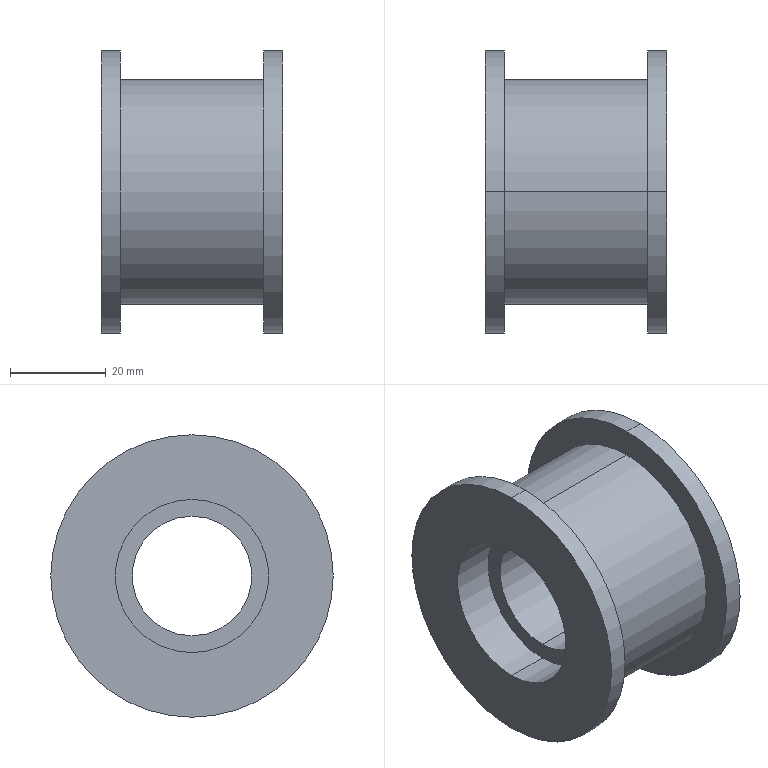Part | STEP file | PN_0041 (slide wheel) | 1 solid | 18 faces | box 38 x 59 x 59 mm | volume 49626 mm3 | cylinder 12 | plane 6 | commonest cylinder face diameters 32 x4 59 x4 25 x2 47 x2
STEP:
#1=CARTESIAN_POINT('',(0.,0.,0.));
#2=DIRECTION('',(0.,0.,1.));
#3=DIRECTION('',(1.,0.,0.));
#4=AXIS2_PLACEMENT_3D('',#1,#2,#3);
#5=CARTESIAN_POINT('',(9.,0.,16.));
#6=VERTEX_POINT('',#5);
#7=CARTESIAN_POINT('',(0.,0.,16.));
#8=VERTEX_POINT('',#7);
#9=CARTESIAN_POINT('',(9.,0.,16.));
#10=DIRECTION('',(-1.,0.,0.));
#11=VECTOR('',#10,1.);
#12=LINE('',#9,#11);
#13=CARTESIAN_POINT('',(9.,0.,0.));
#14=DIRECTION('',(-1.,0.,0.));
#15=DIRECTION('',(0.,0.,1.));
#16=AXIS2_PLACEMENT_3D('',#13,#14,#15);
#17=CYLINDRICAL_SURFACE('',#16,16.);
#18=CARTESIAN_POINT('',(6.283,0.));
#19=DIRECTION('',(0.,1.));
#20=VECTOR('',#19,1.);
#21=LINE('',#18,#20);
#22=(GEOMETRIC_REPRESENTATION_CONTEXT(2)PARAMETRIC_REPRESENTATION_CONTEXT()REPRESENTATION_CONTEXT('',''));
#23=DEFINITIONAL_REPRESENTATION('',(#21),#22);
#24=PCURVE('',#17,#23);
#25=CARTESIAN_POINT('',(9.,0.,0.));
#26=DIRECTION('',(-1.,0.,0.));
#27=DIRECTION('',(0.,0.,1.));
#28=AXIS2_PLACEMENT_3D('',#25,#26,#27);
#29=CYLINDRICAL_SURFACE('',#28,16.);
#30=CARTESIAN_POINT('',(0.,0.));
#31=DIRECTION('',(0.,1.));
#32=VECTOR('',#31,1.);
#33=LINE('',#30,#32);
#34=(GEOMETRIC_REPRESENTATION_CONTEXT(2)PARAMETRIC_REPRESENTATION_CONTEXT()REPRESENTATION_CONTEXT('',''));
#35=DEFINITIONAL_REPRESENTATION('',(#33),#34);
#36=PCURVE('',#29,#35);
#37=SURFACE_CURVE('',#12,(#24,#36),.PCURVE_S1.);
#38=EDGE_CURVE('',#6,#8,#37,.T.);
#39=ORIENTED_EDGE('',*,*,#38,.T.);
#40=CARTESIAN_POINT('',(0.,0.,-16.));
#41=VERTEX_POINT('',#40);
#42=CARTESIAN_POINT('',(0.,0.,0.));
#43=DIRECTION('',(-1.,0.,0.));
#44=DIRECTION('',(0.,0.,1.));
#45=AXIS2_PLACEMENT_3D('',#42,#43,#44);
#46=CIRCLE('',#45,16.);
#47=CARTESIAN_POINT('',(0.,9.));
#48=DIRECTION('',(1.,0.));
#49=VECTOR('',#48,1.);
#50=LINE('',#47,#49);
#51=(GEOMETRIC_REPRESENTATION_CONTEXT(2)PARAMETRIC_REPRESENTATION_CONTEXT()REPRESENTATION_CONTEXT('',''));
#52=DEFINITIONAL_REPRESENTATION('',(#50),#51);
#53=PCURVE('',#17,#52);
#54=CARTESIAN_POINT('',(0.,0.,0.));
#55=DIRECTION('',(1.,0.,0.));
#56=DIRECTION('',(0.,0.,-1.));
#57=AXIS2_PLACEMENT_3D('',#54,#55,#56);
#58=PLANE('',#57);
#59=CARTESIAN_POINT('',(-16.,0.));
#60=CARTESIAN_POINT('',(-16.,27.713));
#61=CARTESIAN_POINT('',(8.,13.856));
#62=CARTESIAN_POINT('',(32.,0.));
#63=CARTESIAN_POINT('',(8.,-13.856));
#64=CARTESIAN_POINT('',(-16.,-27.713));
#65=CARTESIAN_POINT('',(-16.,0.));
#66=(BOUNDED_CURVE()B_SPLINE_CURVE(2,(#59,#60,#61,#62,#63,#64,#65),.UNSPECIFIED.,.T.,.F.)B_SPLINE_CURVE_WITH_KNOTS((1,2,2,2,2,1),(-2.094,0.,2.094,4.189,6.283,8.378),.UNSPECIFIED.)CURVE()GEOMETRIC_REPRESENTATION_ITEM()RATIONAL_B_SPLINE_CURVE((1.,0.5,1.,0.5,1.,0.5,1.))REPRESENTATION_ITEM(''));
#67=(GEOMETRIC_REPRESENTATION_CONTEXT(2)PARAMETRIC_REPRESENTATION_CONTEXT()REPRESENTATION_CONTEXT('',''));
#68=DEFINITIONAL_REPRESENTATION('',(#66),#67);
#69=PCURVE('',#58,#68);
#70=SURFACE_CURVE('',#46,(#53,#69),.PCURVE_S1.);
#71=EDGE_CURVE('',#41,#8,#70,.T.);
#72=ORIENTED_EDGE('',*,*,#71,.F.);
#73=CARTESIAN_POINT('',(9.,0.,-16.));
#74=VERTEX_POINT('',#73);
#75=CARTESIAN_POINT('',(9.,0.,-16.));
#76=DIRECTION('',(-1.,0.,0.));
#77=VECTOR('',#76,1.);
#78=LINE('',#75,#77);
#79=CARTESIAN_POINT('',(3.142,0.));
#80=DIRECTION('',(0.,1.));
#81=VECTOR('',#80,1.);
#82=LINE('',#79,#81);
#83=(GEOMETRIC_REPRESENTATION_CONTEXT(2)PARAMETRIC_REPRESENTATION_CONTEXT()REPRESENTATION_CONTEXT('',''));
#84=DEFINITIONAL_REPRESENTATION('',(#82),#83);
#85=PCURVE('',#17,#84);
#86=CARTESIAN_POINT('',(3.142,0.));
#87=DIRECTION('',(0.,1.));
#88=VECTOR('',#87,1.);
#89=LINE('',#86,#88);
#90=(GEOMETRIC_REPRESENTATION_CONTEXT(2)PARAMETRIC_REPRESENTATION_CONTEXT()REPRESENTATION_CONTEXT('',''));
#91=DEFINITIONAL_REPRESENTATION('',(#89),#90);
#92=PCURVE('',#29,#91);
#93=SURFACE_CURVE('',#78,(#85,#92),.PCURVE_S1.);
#94=EDGE_CURVE('',#74,#41,#93,.T.);
#95=ORIENTED_EDGE('',*,*,#94,.F.);
#96=CARTESIAN_POINT('',(9.,0.,0.));
#97=DIRECTION('',(-1.,0.,0.));
#98=DIRECTION('',(0.,0.,1.));
#99=AXIS2_PLACEMENT_3D('',#96,#97,#98);
#100=CIRCLE('',#99,16.);
#101=CARTESIAN_POINT('',(0.,0.));
#102=DIRECTION('',(1.,0.));
#103=VECTOR('',#102,1.);
#104=LINE('',#101,#103);
#105=(GEOMETRIC_REPRESENTATION_CONTEXT(2)PARAMETRIC_REPRESENTATION_CONTEXT()REPRESENTATION_CONTEXT('',''));
#106=DEFINITIONAL_REPRESENTATION('',(#104),#105);
#107=PCURVE('',#17,#106);
#108=CARTESIAN_POINT('',(9.,0.,0.));
#109=DIRECTION('',(-1.,0.,0.));
#110=DIRECTION('',(0.,0.,1.));
#111=AXIS2_PLACEMENT_3D('',#108,#109,#110);
#112=PLANE('',#111);
#113=CARTESIAN_POINT('',(0.,0.));
#114=DIRECTION('',(1.,0.));
#115=AXIS2_PLACEMENT_2D('',#113,#114);
#116=CIRCLE('',#115,16.);
#117=(GEOMETRIC_REPRESENTATION_CONTEXT(2)PARAMETRIC_REPRESENTATION_CONTEXT()REPRESENTATION_CONTEXT('',''));
#118=DEFINITIONAL_REPRESENTATION('',(#116),#117);
#119=PCURVE('',#112,#118);
#120=SURFACE_CURVE('',#100,(#107,#119),.PCURVE_S1.);
#121=EDGE_CURVE('',#74,#6,#120,.T.);
#122=ORIENTED_EDGE('',*,*,#121,.T.);
#123=EDGE_LOOP('',(#39,#72,#95,#122));
#124=FACE_BOUND('',#123,.F.);
#125=ADVANCED_FACE('',(#124),#17,.F.);
#126=CARTESIAN_POINT('',(29.,0.,-16.));
#127=VERTEX_POINT('',#126);
#128=CARTESIAN_POINT('',(38.,0.,-16.));
#129=VERTEX_POINT('',#128);
#130=CARTESIAN_POINT('',(29.,0.,-16.));
#131=DIRECTION('',(1.,0.,0.));
#132=VECTOR('',#131,1.);
#133=LINE('',#130,#132);
#134=CARTESIAN_POINT('',(29.,0.,0.));
#135=DIRECTION('',(1.,0.,0.));
#136=DIRECTION('',(0.,0.,-1.));
#137=AXIS2_PLACEMENT_3D('',#134,#135,#136);
#138=CYLINDRICAL_SURFACE('',#137,16.);
#139=CARTESIAN_POINT('',(6.283,0.));
#140=DIRECTION('',(0.,1.));
#141=VECTOR('',#140,1.);
#142=LINE('',#139,#141);
#143=(GEOMETRIC_REPRESENTATION_CONTEXT(2)PARAMETRIC_REPRESENTATION_CONTEXT()REPRESENTATION_CONTEXT('',''));
#144=DEFINITIONAL_REPRESENTATION('',(#142),#143);
#145=PCURVE('',#138,#144);
#146=CARTESIAN_POINT('',(29.,0.,0.));
#147=DIRECTION('',(1.,0.,0.));
#148=DIRECTION('',(0.,0.,-1.));
#149=AXIS2_PLACEMENT_3D('',#146,#147,#148);
#150=CYLINDRICAL_SURFACE('',#149,16.);
#151=CARTESIAN_POINT('',(0.,0.));
#152=DIRECTION('',(0.,1.));
#153=VECTOR('',#152,1.);
#154=LINE('',#151,#153);
#155=(GEOMETRIC_REPRESENTATION_CONTEXT(2)PARAMETRIC_REPRESENTATION_CONTEXT()REPRESENTATION_CONTEXT('',''));
#156=DEFINITIONAL_REPRESENTATION('',(#154),#155);
#157=PCURVE('',#150,#156);
#158=SURFACE_CURVE('',#133,(#145,#157),.PCURVE_S1.);
#159=EDGE_CURVE('',#127,#129,#158,.T.);
#160=ORIENTED_EDGE('',*,*,#159,.T.);
#161=CARTESIAN_POINT('',(38.,0.,16.));
#162=VERTEX_POINT('',#161);
#163=CARTESIAN_POINT('',(38.,0.,0.));
#164=DIRECTION('',(1.,0.,0.));
#165=DIRECTION('',(0.,0.,-1.));
#166=AXIS2_PLACEMENT_3D('',#163,#164,#165);
#167=CIRCLE('',#166,16.);
#168=CARTESIAN_POINT('',(0.,9.));
#169=DIRECTION('',(1.,0.));
#170=VECTOR('',#169,1.);
#171=LINE('',#168,#170);
#172=(GEOMETRIC_REPRESENTATION_CONTEXT(2)PARAMETRIC_REPRESENTATION_CONTEXT()REPRESENTATION_CONTEXT('',''));
#173=DEFINITIONAL_REPRESENTATION('',(#171),#172);
#174=PCURVE('',#138,#173);
#175=CARTESIAN_POINT('',(38.,29.5,0.));
#176=DIRECTION('',(-1.,0.,0.));
#177=DIRECTION('',(0.,0.,1.));
#178=AXIS2_PLACEMENT_3D('',#175,#176,#177);
#179=PLANE('',#178);
#180=CARTESIAN_POINT('',(-16.,-29.5));
#181=CARTESIAN_POINT('',(-16.,-1.787));
#182=CARTESIAN_POINT('',(8.,-15.644));
#183=CARTESIAN_POINT('',(32.,-29.5));
#184=CARTESIAN_POINT('',(8.,-43.356));
#185=CARTESIAN_POINT('',(-16.,-57.213));
#186=CARTESIAN_POINT('',(-16.,-29.5));
#187=(BOUNDED_CURVE()B_SPLINE_CURVE(2,(#180,#181,#182,#183,#184,#185,#186),.UNSPECIFIED.,.T.,.F.)B_SPLINE_CURVE_WITH_KNOTS((1,2,2,2,2,1),(-2.094,0.,2.094,4.189,6.283,8.378),.UNSPECIFIED.)CURVE()GEOMETRIC_REPRESENTATION_ITEM()RATIONAL_B_SPLINE_CURVE((1.,0.5,1.,0.5,1.,0.5,1.))REPRESENTATION_ITEM(''));
#188=(GEOMETRIC_REPRESENTATION_CONTEXT(2)PARAMETRIC_REPRESENTATION_CONTEXT()REPRESENTATION_CONTEXT('',''));
#189=DEFINITIONAL_REPRESENTATION('',(#187),#188);
#190=PCURVE('',#179,#189);
#191=SURFACE_CURVE('',#167,(#174,#190),.PCURVE_S1.);
#192=EDGE_CURVE('',#162,#129,#191,.T.);
#193=ORIENTED_EDGE('',*,*,#192,.F.);
#194=CARTESIAN_POINT('',(29.,0.,16.));
#195=VERTEX_POINT('',#194);
#196=CARTESIAN_POINT('',(29.,0.,16.));
#197=DIRECTION('',(1.,0.,0.));
#198=VECTOR('',#197,1.);
#199=LINE('',#196,#198);
#200=CARTESIAN_POINT('',(3.142,0.));
#201=DIRECTION('',(0.,1.));
#202=VECTOR('',#201,1.);
#203=LINE('',#200,#202);
#204=(GEOMETRIC_REPRESENTATION_CONTEXT(2)PARAMETRIC_REPRESENTATION_CONTEXT()REPRESENTATION_CONTEXT('',''));
#205=DEFINITIONAL_REPRESENTATION('',(#203),#204);
#206=PCURVE('',#138,#205);
#207=CARTESIAN_POINT('',(3.142,0.));
#208=DIRECTION('',(0.,1.));
#209=VECTOR('',#208,1.);
#210=LINE('',#207,#209);
#211=(GEOMETRIC_REPRESENTATION_CONTEXT(2)PARAMETRIC_REPRESENTATION_CONTEXT()REPRESENTATION_CONTEXT('',''));
#212=DEFINITIONAL_REPRESENTATION('',(#210),#211);
#213=PCURVE('',#150,#212);
#214=SURFACE_CURVE('',#199,(#206,#213),.PCURVE_S1.);
#215=EDGE_CURVE('',#195,#162,#214,.T.);
#216=ORIENTED_EDGE('',*,*,#215,.F.);
#217=CARTESIAN_POINT('',(29.,0.,0.));
#218=DIRECTION('',(1.,0.,0.));
#219=DIRECTION('',(0.,0.,-1.));
#220=AXIS2_PLACEMENT_3D('',#217,#218,#219);
#221=CIRCLE('',#220,16.);
#222=CARTESIAN_POINT('',(0.,0.));
#223=DIRECTION('',(1.,0.));
#224=VECTOR('',#223,1.);
#225=LINE('',#222,#224);
#226=(GEOMETRIC_REPRESENTATION_CONTEXT(2)PARAMETRIC_REPRESENTATION_CONTEXT()REPRESENTATION_CONTEXT('',''));
#227=DEFINITIONAL_REPRESENTATION('',(#225),#226);
#228=PCURVE('',#138,#227);
#229=CARTESIAN_POINT('',(29.,0.,0.));
#230=DIRECTION('',(1.,0.,0.));
#231=DIRECTION('',(0.,0.,-1.));
#232=AXIS2_PLACEMENT_3D('',#229,#230,#231);
#233=PLANE('',#232);
#234=CARTESIAN_POINT('',(0.,0.));
#235=DIRECTION('',(1.,0.));
#236=AXIS2_PLACEMENT_2D('',#234,#235);
#237=CIRCLE('',#236,16.);
#238=(GEOMETRIC_REPRESENTATION_CONTEXT(2)PARAMETRIC_REPRESENTATION_CONTEXT()REPRESENTATION_CONTEXT('',''));
#239=DEFINITIONAL_REPRESENTATION('',(#237),#238);
#240=PCURVE('',#233,#239);
#241=SURFACE_CURVE('',#221,(#228,#240),.PCURVE_S1.);
#242=EDGE_CURVE('',#195,#127,#241,.T.);
#243=ORIENTED_EDGE('',*,*,#242,.T.);
#244=EDGE_LOOP('',(#160,#193,#216,#243));
#245=FACE_BOUND('',#244,.F.);
#246=ADVANCED_FACE('',(#245),#138,.F.);
#247=CARTESIAN_POINT('',(38.,0.,29.5));
#248=VERTEX_POINT('',#247);
#249=CARTESIAN_POINT('',(38.,0.,-29.5));
#250=VERTEX_POINT('',#249);
#251=CARTESIAN_POINT('',(38.,0.,0.));
#252=DIRECTION('',(-1.,0.,0.));
#253=DIRECTION('',(0.,0.,1.));
#254=AXIS2_PLACEMENT_3D('',#251,#252,#253);
#255=CIRCLE('',#254,29.5);
#256=CARTESIAN_POINT('',(0.,0.,0.));
#257=DIRECTION('',(-1.,0.,0.));
#258=DIRECTION('',(0.,0.,1.));
#259=AXIS2_PLACEMENT_3D('',#256,#257,#258);
#260=CYLINDRICAL_SURFACE('',#259,29.5);
#261=CARTESIAN_POINT('',(0.,-38.));
#262=DIRECTION('',(1.,0.));
#263=VECTOR('',#262,1.);
#264=LINE('',#261,#263);
#265=(GEOMETRIC_REPRESENTATION_CONTEXT(2)PARAMETRIC_REPRESENTATION_CONTEXT()REPRESENTATION_CONTEXT('',''));
#266=DEFINITIONAL_REPRESENTATION('',(#264),#265);
#267=PCURVE('',#260,#266);
#268=CARTESIAN_POINT('',(0.,-29.5));
#269=DIRECTION('',(1.,0.));
#270=AXIS2_PLACEMENT_2D('',#268,#269);
#271=CIRCLE('',#270,29.5);
#272=(GEOMETRIC_REPRESENTATION_CONTEXT(2)PARAMETRIC_REPRESENTATION_CONTEXT()REPRESENTATION_CONTEXT('',''));
#273=DEFINITIONAL_REPRESENTATION('',(#271),#272);
#274=PCURVE('',#179,#273);
#275=SURFACE_CURVE('',#255,(#267,#274),.PCURVE_S1.);
#276=EDGE_CURVE('',#248,#250,#275,.T.);
#277=ORIENTED_EDGE('',*,*,#276,.T.);
#278=CARTESIAN_POINT('',(34.,0.,-29.5));
#279=VERTEX_POINT('',#278);
#280=CARTESIAN_POINT('',(0.,0.,-29.5));
#281=DIRECTION('',(-1.,0.,0.));
#282=VECTOR('',#281,1.);
#283=LINE('',#280,#282);
#284=CARTESIAN_POINT('',(3.142,0.));
#285=DIRECTION('',(0.,1.));
#286=VECTOR('',#285,1.);
#287=LINE('',#284,#286);
#288=(GEOMETRIC_REPRESENTATION_CONTEXT(2)PARAMETRIC_REPRESENTATION_CONTEXT()REPRESENTATION_CONTEXT('',''));
#289=DEFINITIONAL_REPRESENTATION('',(#287),#288);
#290=PCURVE('',#260,#289);
#291=CARTESIAN_POINT('',(0.,0.,0.));
#292=DIRECTION('',(-1.,0.,0.));
#293=DIRECTION('',(0.,0.,1.));
#294=AXIS2_PLACEMENT_3D('',#291,#292,#293);
#295=CYLINDRICAL_SURFACE('',#294,29.5);
#296=CARTESIAN_POINT('',(3.142,0.));
#297=DIRECTION('',(0.,1.));
#298=VECTOR('',#297,1.);
#299=LINE('',#296,#298);
#300=(GEOMETRIC_REPRESENTATION_CONTEXT(2)PARAMETRIC_REPRESENTATION_CONTEXT()REPRESENTATION_CONTEXT('',''));
#301=DEFINITIONAL_REPRESENTATION('',(#299),#300);
#302=PCURVE('',#295,#301);
#303=SURFACE_CURVE('',#283,(#290,#302),.PCURVE_S1.);
#304=EDGE_CURVE('',#250,#279,#303,.T.);
#305=ORIENTED_EDGE('',*,*,#304,.T.);
#306=CARTESIAN_POINT('',(34.,0.,29.5));
#307=VERTEX_POINT('',#306);
#308=CARTESIAN_POINT('',(34.,0.,0.));
#309=DIRECTION('',(-1.,0.,0.));
#310=DIRECTION('',(0.,0.,1.));
#311=AXIS2_PLACEMENT_3D('',#308,#309,#310);
#312=CIRCLE('',#311,29.5);
#313=CARTESIAN_POINT('',(0.,-34.));
#314=DIRECTION('',(1.,0.));
#315=VECTOR('',#314,1.);
#316=LINE('',#313,#315);
#317=(GEOMETRIC_REPRESENTATION_CONTEXT(2)PARAMETRIC_REPRESENTATION_CONTEXT()REPRESENTATION_CONTEXT('',''));
#318=DEFINITIONAL_REPRESENTATION('',(#316),#317);
#319=PCURVE('',#260,#318);
#320=CARTESIAN_POINT('',(34.,23.5,0.));
#321=DIRECTION('',(1.,0.,0.));
#322=DIRECTION('',(0.,0.,-1.));
#323=AXIS2_PLACEMENT_3D('',#320,#321,#322);
#324=PLANE('',#323);
#325=CARTESIAN_POINT('',(-29.5,-23.5));
#326=CARTESIAN_POINT('',(-29.5,27.595));
#327=CARTESIAN_POINT('',(14.75,2.048));
#328=CARTESIAN_POINT('',(59.,-23.5));
#329=CARTESIAN_POINT('',(14.75,-49.048));
#330=CARTESIAN_POINT('',(-29.5,-74.595));
#331=CARTESIAN_POINT('',(-29.5,-23.5));
#332=(BOUNDED_CURVE()B_SPLINE_CURVE(2,(#325,#326,#327,#328,#329,#330,#331),.UNSPECIFIED.,.T.,.F.)B_SPLINE_CURVE_WITH_KNOTS((1,2,2,2,2,1),(-2.094,0.,2.094,4.189,6.283,8.378),.UNSPECIFIED.)CURVE()GEOMETRIC_REPRESENTATION_ITEM()RATIONAL_B_SPLINE_CURVE((1.,0.5,1.,0.5,1.,0.5,1.))REPRESENTATION_ITEM(''));
#333=(GEOMETRIC_REPRESENTATION_CONTEXT(2)PARAMETRIC_REPRESENTATION_CONTEXT()REPRESENTATION_CONTEXT('',''));
#334=DEFINITIONAL_REPRESENTATION('',(#332),#333);
#335=PCURVE('',#324,#334);
#336=SURFACE_CURVE('',#312,(#319,#335),.PCURVE_S1.);
#337=EDGE_CURVE('',#307,#279,#336,.T.);
#338=ORIENTED_EDGE('',*,*,#337,.F.);
#339=CARTESIAN_POINT('',(0.,0.,29.5));
#340=DIRECTION('',(-1.,0.,0.));
#341=VECTOR('',#340,1.);
#342=LINE('',#339,#341);
#343=CARTESIAN_POINT('',(0.,0.));
#344=DIRECTION('',(0.,1.));
#345=VECTOR('',#344,1.);
#346=LINE('',#343,#345);
#347=(GEOMETRIC_REPRESENTATION_CONTEXT(2)PARAMETRIC_REPRESENTATION_CONTEXT()REPRESENTATION_CONTEXT('',''));
#348=DEFINITIONAL_REPRESENTATION('',(#346),#347);
#349=PCURVE('',#260,#348);
#350=CARTESIAN_POINT('',(6.283,0.));
#351=DIRECTION('',(0.,1.));
#352=VECTOR('',#351,1.);
#353=LINE('',#350,#352);
#354=(GEOMETRIC_REPRESENTATION_CONTEXT(2)PARAMETRIC_REPRESENTATION_CONTEXT()REPRESENTATION_CONTEXT('',''));
#355=DEFINITIONAL_REPRESENTATION('',(#353),#354);
#356=PCURVE('',#295,#355);
#357=SURFACE_CURVE('',#342,(#349,#356),.PCURVE_S1.);
#358=EDGE_CURVE('',#248,#307,#357,.T.);
#359=ORIENTED_EDGE('',*,*,#358,.F.);
#360=EDGE_LOOP('',(#277,#305,#338,#359));
#361=FACE_BOUND('',#360,.T.);
#362=ADVANCED_FACE('',(#361),#260,.T.);
#363=CARTESIAN_POINT('',(34.,0.,23.5));
#364=VERTEX_POINT('',#363);
#365=CARTESIAN_POINT('',(34.,0.,-23.5));
#366=VERTEX_POINT('',#365);
#367=CARTESIAN_POINT('',(34.,0.,0.));
#368=DIRECTION('',(-1.,0.,0.));
#369=DIRECTION('',(0.,0.,1.));
#370=AXIS2_PLACEMENT_3D('',#367,#368,#369);
#371=CIRCLE('',#370,23.5);
#372=CARTESIAN_POINT('',(0.,0.,0.));
#373=DIRECTION('',(-1.,0.,0.));
#374=DIRECTION('',(0.,0.,1.));
#375=AXIS2_PLACEMENT_3D('',#372,#373,#374);
#376=CYLINDRICAL_SURFACE('',#375,23.5);
#377=CARTESIAN_POINT('',(0.,-34.));
#378=DIRECTION('',(1.,0.));
#379=VECTOR('',#378,1.);
#380=LINE('',#377,#379);
#381=(GEOMETRIC_REPRESENTATION_CONTEXT(2)PARAMETRIC_REPRESENTATION_CONTEXT()REPRESENTATION_CONTEXT('',''));
#382=DEFINITIONAL_REPRESENTATION('',(#380),#381);
#383=PCURVE('',#376,#382);
#384=CARTESIAN_POINT('',(-23.5,-23.5));
#385=CARTESIAN_POINT('',(-23.5,17.203));
#386=CARTESIAN_POINT('',(11.75,-3.148));
#387=CARTESIAN_POINT('',(47.,-23.5));
#388=CARTESIAN_POINT('',(11.75,-43.852));
#389=CARTESIAN_POINT('',(-23.5,-64.203));
#390=CARTESIAN_POINT('',(-23.5,-23.5));
#391=(BOUNDED_CURVE()B_SPLINE_CURVE(2,(#384,#385,#386,#387,#388,#389,#390),.UNSPECIFIED.,.T.,.F.)B_SPLINE_CURVE_WITH_KNOTS((1,2,2,2,2,1),(-2.094,0.,2.094,4.189,6.283,8.378),.UNSPECIFIED.)CURVE()GEOMETRIC_REPRESENTATION_ITEM()RATIONAL_B_SPLINE_CURVE((1.,0.5,1.,0.5,1.,0.5,1.))REPRESENTATION_ITEM(''));
#392=(GEOMETRIC_REPRESENTATION_CONTEXT(2)PARAMETRIC_REPRESENTATION_CONTEXT()REPRESENTATION_CONTEXT('',''));
#393=DEFINITIONAL_REPRESENTATION('',(#391),#392);
#394=PCURVE('',#324,#393);
#395=SURFACE_CURVE('',#371,(#383,#394),.PCURVE_S1.);
#396=EDGE_CURVE('',#364,#366,#395,.T.);
#397=ORIENTED_EDGE('',*,*,#396,.T.);
#398=CARTESIAN_POINT('',(4.,0.,-23.5));
#399=VERTEX_POINT('',#398);
#400=CARTESIAN_POINT('',(0.,0.,-23.5));
#401=DIRECTION('',(-1.,0.,0.));
#402=VECTOR('',#401,1.);
#403=LINE('',#400,#402);
#404=CARTESIAN_POINT('',(3.142,0.));
#405=DIRECTION('',(0.,1.));
#406=VECTOR('',#405,1.);
#407=LINE('',#404,#406);
#408=(GEOMETRIC_REPRESENTATION_CONTEXT(2)PARAMETRIC_REPRESENTATION_CONTEXT()REPRESENTATION_CONTEXT('',''));
#409=DEFINITIONAL_REPRESENTATION('',(#407),#408);
#410=PCURVE('',#376,#409);
#411=CARTESIAN_POINT('',(0.,0.,0.));
#412=DIRECTION('',(-1.,0.,0.));
#413=DIRECTION('',(0.,0.,1.));
#414=AXIS2_PLACEMENT_3D('',#411,#412,#413);
#415=CYLINDRICAL_SURFACE('',#414,23.5);
#416=CARTESIAN_POINT('',(3.142,0.));
#417=DIRECTION('',(0.,1.));
#418=VECTOR('',#417,1.);
#419=LINE('',#416,#418);
#420=(GEOMETRIC_REPRESENTATION_CONTEXT(2)PARAMETRIC_REPRESENTATION_CONTEXT()REPRESENTATION_CONTEXT('',''));
#421=DEFINITIONAL_REPRESENTATION('',(#419),#420);
#422=PCURVE('',#415,#421);
#423=SURFACE_CURVE('',#403,(#410,#422),.PCURVE_S1.);
#424=EDGE_CURVE('',#366,#399,#423,.T.);
#425=ORIENTED_EDGE('',*,*,#424,.T.);
#426=CARTESIAN_POINT('',(4.,0.,23.5));
#427=VERTEX_POINT('',#426);
#428=CARTESIAN_POINT('',(4.,0.,0.));
#429=DIRECTION('',(-1.,0.,0.));
#430=DIRECTION('',(0.,0.,1.));
#431=AXIS2_PLACEMENT_3D('',#428,#429,#430);
#432=CIRCLE('',#431,23.5);
#433=CARTESIAN_POINT('',(0.,-4.));
#434=DIRECTION('',(1.,0.));
#435=VECTOR('',#434,1.);
#436=LINE('',#433,#435);
#437=(GEOMETRIC_REPRESENTATION_CONTEXT(2)PARAMETRIC_REPRESENTATION_CONTEXT()REPRESENTATION_CONTEXT('',''));
#438=DEFINITIONAL_REPRESENTATION('',(#436),#437);
#439=PCURVE('',#376,#438);
#440=CARTESIAN_POINT('',(4.,29.5,0.));
#441=DIRECTION('',(-1.,0.,0.));
#442=DIRECTION('',(0.,0.,1.));
#443=AXIS2_PLACEMENT_3D('',#440,#441,#442);
#444=PLANE('',#443);
#445=CARTESIAN_POINT('',(0.,-29.5));
#446=DIRECTION('',(1.,0.));
#447=AXIS2_PLACEMENT_2D('',#445,#446);
#448=CIRCLE('',#447,23.5);
#449=(GEOMETRIC_REPRESENTATION_CONTEXT(2)PARAMETRIC_REPRESENTATION_CONTEXT()REPRESENTATION_CONTEXT('',''));
#450=DEFINITIONAL_REPRESENTATION('',(#448),#449);
#451=PCURVE('',#444,#450);
#452=SURFACE_CURVE('',#432,(#439,#451),.PCURVE_S1.);
#453=EDGE_CURVE('',#427,#399,#452,.T.);
#454=ORIENTED_EDGE('',*,*,#453,.F.);
#455=CARTESIAN_POINT('',(0.,0.,23.5));
#456=DIRECTION('',(-1.,0.,0.));
#457=VECTOR('',#456,1.);
#458=LINE('',#455,#457);
#459=CARTESIAN_POINT('',(0.,0.));
#460=DIRECTION('',(0.,1.));
#461=VECTOR('',#460,1.);
#462=LINE('',#459,#461);
#463=(GEOMETRIC_REPRESENTATION_CONTEXT(2)PARAMETRIC_REPRESENTATION_CONTEXT()REPRESENTATION_CONTEXT('',''));
#464=DEFINITIONAL_REPRESENTATION('',(#462),#463);
#465=PCURVE('',#376,#464);
#466=CARTESIAN_POINT('',(6.283,0.));
#467=DIRECTION('',(0.,1.));
#468=VECTOR('',#467,1.);
#469=LINE('',#466,#468);
#470=(GEOMETRIC_REPRESENTATION_CONTEXT(2)PARAMETRIC_REPRESENTATION_CONTEXT()REPRESENTATION_CONTEXT('',''));
#471=DEFINITIONAL_REPRESENTATION('',(#469),#470);
#472=PCURVE('',#415,#471);
#473=SURFACE_CURVE('',#458,(#465,#472),.PCURVE_S1.);
#474=EDGE_CURVE('',#364,#427,#473,.T.);
#475=ORIENTED_EDGE('',*,*,#474,.F.);
#476=EDGE_LOOP('',(#397,#425,#454,#475));
#477=FACE_BOUND('',#476,.T.);
#478=ADVANCED_FACE('',(#477),#376,.T.);
#479=CARTESIAN_POINT('',(4.,0.,29.5));
#480=VERTEX_POINT('',#479);
#481=CARTESIAN_POINT('',(4.,0.,-29.5));
#482=VERTEX_POINT('',#481);
#483=CARTESIAN_POINT('',(4.,0.,0.));
#484=DIRECTION('',(-1.,0.,0.));
#485=DIRECTION('',(0.,0.,1.));
#486=AXIS2_PLACEMENT_3D('',#483,#484,#485);
#487=CIRCLE('',#486,29.5);
#488=CARTESIAN_POINT('',(0.,0.,0.));
#489=DIRECTION('',(-1.,0.,0.));
#490=DIRECTION('',(0.,0.,1.));
#491=AXIS2_PLACEMENT_3D('',#488,#489,#490);
#492=CYLINDRICAL_SURFACE('',#491,29.5);
#493=CARTESIAN_POINT('',(0.,-4.));
#494=DIRECTION('',(1.,0.));
#495=VECTOR('',#494,1.);
#496=LINE('',#493,#495);
#497=(GEOMETRIC_REPRESENTATION_CONTEXT(2)PARAMETRIC_REPRESENTATION_CONTEXT()REPRESENTATION_CONTEXT('',''));
#498=DEFINITIONAL_REPRESENTATION('',(#496),#497);
#499=PCURVE('',#492,#498);
#500=CARTESIAN_POINT('',(0.,-29.5));
#501=DIRECTION('',(1.,0.));
#502=AXIS2_PLACEMENT_2D('',#500,#501);
#503=CIRCLE('',#502,29.5);
#504=(GEOMETRIC_REPRESENTATION_CONTEXT(2)PARAMETRIC_REPRESENTATION_CONTEXT()REPRESENTATION_CONTEXT('',''));
#505=DEFINITIONAL_REPRESENTATION('',(#503),#504);
#506=PCURVE('',#444,#505);
#507=SURFACE_CURVE('',#487,(#499,#506),.PCURVE_S1.);
#508=EDGE_CURVE('',#480,#482,#507,.T.);
#509=ORIENTED_EDGE('',*,*,#508,.T.);
#510=CARTESIAN_POINT('',(0.,0.,-29.5));
#511=VERTEX_POINT('',#510);
#512=CARTESIAN_POINT('',(0.,0.,-29.5));
#513=DIRECTION('',(-1.,0.,0.));
#514=VECTOR('',#513,1.);
#515=LINE('',#512,#514);
#516=CARTESIAN_POINT('',(3.142,0.));
#517=DIRECTION('',(0.,1.));
#518=VECTOR('',#517,1.);
#519=LINE('',#516,#518);
#520=(GEOMETRIC_REPRESENTATION_CONTEXT(2)PARAMETRIC_REPRESENTATION_CONTEXT()REPRESENTATION_CONTEXT('',''));
#521=DEFINITIONAL_REPRESENTATION('',(#519),#520);
#522=PCURVE('',#492,#521);
#523=CARTESIAN_POINT('',(0.,0.,0.));
#524=DIRECTION('',(-1.,0.,0.));
#525=DIRECTION('',(0.,0.,1.));
#526=AXIS2_PLACEMENT_3D('',#523,#524,#525);
#527=CYLINDRICAL_SURFACE('',#526,29.5);
#528=CARTESIAN_POINT('',(3.142,0.));
#529=DIRECTION('',(0.,1.));
#530=VECTOR('',#529,1.);
#531=LINE('',#528,#530);
#532=(GEOMETRIC_REPRESENTATION_CONTEXT(2)PARAMETRIC_REPRESENTATION_CONTEXT()REPRESENTATION_CONTEXT('',''));
#533=DEFINITIONAL_REPRESENTATION('',(#531),#532);
#534=PCURVE('',#527,#533);
#535=SURFACE_CURVE('',#515,(#522,#534),.PCURVE_S1.);
#536=EDGE_CURVE('',#482,#511,#535,.T.);
#537=ORIENTED_EDGE('',*,*,#536,.T.);
#538=CARTESIAN_POINT('',(0.,0.,29.5));
#539=VERTEX_POINT('',#538);
#540=CARTESIAN_POINT('',(0.,0.,0.));
#541=DIRECTION('',(-1.,0.,0.));
#542=DIRECTION('',(0.,0.,1.));
#543=AXIS2_PLACEMENT_3D('',#540,#541,#542);
#544=CIRCLE('',#543,29.5);
#545=CARTESIAN_POINT('',(0.,0.));
#546=DIRECTION('',(1.,0.));
#547=VECTOR('',#546,1.);
#548=LINE('',#545,#547);
#549=(GEOMETRIC_REPRESENTATION_CONTEXT(2)PARAMETRIC_REPRESENTATION_CONTEXT()REPRESENTATION_CONTEXT('',''));
#550=DEFINITIONAL_REPRESENTATION('',(#548),#549);
#551=PCURVE('',#492,#550);
#552=CARTESIAN_POINT('',(-29.5,0.));
#553=CARTESIAN_POINT('',(-29.5,51.095));
#554=CARTESIAN_POINT('',(14.75,25.548));
#555=CARTESIAN_POINT('',(59.,0.));
#556=CARTESIAN_POINT('',(14.75,-25.548));
#557=CARTESIAN_POINT('',(-29.5,-51.095));
#558=CARTESIAN_POINT('',(-29.5,0.));
#559=(BOUNDED_CURVE()B_SPLINE_CURVE(2,(#552,#553,#554,#555,#556,#557,#558),.UNSPECIFIED.,.T.,.F.)B_SPLINE_CURVE_WITH_KNOTS((1,2,2,2,2,1),(-2.094,0.,2.094,4.189,6.283,8.378),.UNSPECIFIED.)CURVE()GEOMETRIC_REPRESENTATION_ITEM()RATIONAL_B_SPLINE_CURVE((1.,0.5,1.,0.5,1.,0.5,1.))REPRESENTATION_ITEM(''));
#560=(GEOMETRIC_REPRESENTATION_CONTEXT(2)PARAMETRIC_REPRESENTATION_CONTEXT()REPRESENTATION_CONTEXT('',''));
#561=DEFINITIONAL_REPRESENTATION('',(#559),#560);
#562=PCURVE('',#58,#561);
#563=SURFACE_CURVE('',#544,(#551,#562),.PCURVE_S1.);
#564=EDGE_CURVE('',#539,#511,#563,.T.);
#565=ORIENTED_EDGE('',*,*,#564,.F.);
#566=CARTESIAN_POINT('',(0.,0.,29.5));
#567=DIRECTION('',(-1.,0.,0.));
#568=VECTOR('',#567,1.);
#569=LINE('',#566,#568);
#570=CARTESIAN_POINT('',(0.,0.));
#571=DIRECTION('',(0.,1.));
#572=VECTOR('',#571,1.);
#573=LINE('',#570,#572);
#574=(GEOMETRIC_REPRESENTATION_CONTEXT(2)PARAMETRIC_REPRESENTATION_CONTEXT()REPRESENTATION_CONTEXT('',''));
#575=DEFINITIONAL_REPRESENTATION('',(#573),#574);
#576=PCURVE('',#492,#575);
#577=CARTESIAN_POINT('',(6.283,0.));
#578=DIRECTION('',(0.,1.));
#579=VECTOR('',#578,1.);
#580=LINE('',#577,#579);
#581=(GEOMETRIC_REPRESENTATION_CONTEXT(2)PARAMETRIC_REPRESENTATION_CONTEXT()REPRESENTATION_CONTEXT('',''));
#582=DEFINITIONAL_REPRESENTATION('',(#580),#581);
#583=PCURVE('',#527,#582);
#584=SURFACE_CURVE('',#569,(#576,#583),.PCURVE_S1.);
#585=EDGE_CURVE('',#480,#539,#584,.T.);
#586=ORIENTED_EDGE('',*,*,#585,.F.);
#587=EDGE_LOOP('',(#509,#537,#565,#586));
#588=FACE_BOUND('',#587,.T.);
#589=ADVANCED_FACE('',(#588),#492,.T.);
#590=CARTESIAN_POINT('',(9.,0.,-12.5));
#591=VERTEX_POINT('',#590);
#592=CARTESIAN_POINT('',(29.,0.,-12.5));
#593=VERTEX_POINT('',#592);
#594=CARTESIAN_POINT('',(0.,0.,-12.5));
#595=DIRECTION('',(1.,0.,0.));
#596=VECTOR('',#595,1.);
#597=LINE('',#594,#596);
#598=CARTESIAN_POINT('',(0.,0.,0.));
#599=DIRECTION('',(1.,0.,0.));
#600=DIRECTION('',(0.,0.,-1.));
#601=AXIS2_PLACEMENT_3D('',#598,#599,#600);
#602=CYLINDRICAL_SURFACE('',#601,12.5);
#603=CARTESIAN_POINT('',(6.283,0.));
#604=DIRECTION('',(0.,1.));
#605=VECTOR('',#604,1.);
#606=LINE('',#603,#605);
#607=(GEOMETRIC_REPRESENTATION_CONTEXT(2)PARAMETRIC_REPRESENTATION_CONTEXT()REPRESENTATION_CONTEXT('',''));
#608=DEFINITIONAL_REPRESENTATION('',(#606),#607);
#609=PCURVE('',#602,#608);
#610=CARTESIAN_POINT('',(0.,0.,0.));
#611=DIRECTION('',(1.,0.,0.));
#612=DIRECTION('',(0.,0.,-1.));
#613=AXIS2_PLACEMENT_3D('',#610,#611,#612);
#614=CYLINDRICAL_SURFACE('',#613,12.5);
#615=CARTESIAN_POINT('',(0.,0.));
#616=DIRECTION('',(0.,1.));
#617=VECTOR('',#616,1.);
#618=LINE('',#615,#617);
#619=(GEOMETRIC_REPRESENTATION_CONTEXT(2)PARAMETRIC_REPRESENTATION_CONTEXT()REPRESENTATION_CONTEXT('',''));
#620=DEFINITIONAL_REPRESENTATION('',(#618),#619);
#621=PCURVE('',#614,#620);
#622=SURFACE_CURVE('',#597,(#609,#621),.PCURVE_S1.);
#623=EDGE_CURVE('',#591,#593,#622,.T.);
#624=ORIENTED_EDGE('',*,*,#623,.T.);
#625=CARTESIAN_POINT('',(29.,0.,12.5));
#626=VERTEX_POINT('',#625);
#627=CARTESIAN_POINT('',(29.,0.,0.));
#628=DIRECTION('',(-1.,0.,0.));
#629=DIRECTION('',(0.,0.,-1.));
#630=AXIS2_PLACEMENT_3D('',#627,#628,#629);
#631=CIRCLE('',#630,12.5);
#632=CARTESIAN_POINT('',(6.283,29.));
#633=DIRECTION('',(-1.,0.));
#634=VECTOR('',#633,1.);
#635=LINE('',#632,#634);
#636=(GEOMETRIC_REPRESENTATION_CONTEXT(2)PARAMETRIC_REPRESENTATION_CONTEXT()REPRESENTATION_CONTEXT('',''));
#637=DEFINITIONAL_REPRESENTATION('',(#635),#636);
#638=PCURVE('',#602,#637);
#639=CARTESIAN_POINT('',(12.5,0.));
#640=CARTESIAN_POINT('',(12.5,-21.651));
#641=CARTESIAN_POINT('',(-6.25,-10.825));
#642=CARTESIAN_POINT('',(-25.,0.));
#643=CARTESIAN_POINT('',(-6.25,10.825));
#644=CARTESIAN_POINT('',(12.5,21.651));
#645=CARTESIAN_POINT('',(12.5,0.));
#646=(BOUNDED_CURVE()B_SPLINE_CURVE(2,(#639,#640,#641,#642,#643,#644,#645),.UNSPECIFIED.,.T.,.F.)B_SPLINE_CURVE_WITH_KNOTS((1,2,2,2,2,1),(-2.094,0.,2.094,4.189,6.283,8.378),.UNSPECIFIED.)CURVE()GEOMETRIC_REPRESENTATION_ITEM()RATIONAL_B_SPLINE_CURVE((1.,0.5,1.,0.5,1.,0.5,1.))REPRESENTATION_ITEM(''));
#647=(GEOMETRIC_REPRESENTATION_CONTEXT(2)PARAMETRIC_REPRESENTATION_CONTEXT()REPRESENTATION_CONTEXT('',''));
#648=DEFINITIONAL_REPRESENTATION('',(#646),#647);
#649=PCURVE('',#233,#648);
#650=SURFACE_CURVE('',#631,(#638,#649),.PCURVE_S1.);
#651=EDGE_CURVE('',#593,#626,#650,.T.);
#652=ORIENTED_EDGE('',*,*,#651,.T.);
#653=CARTESIAN_POINT('',(9.,0.,12.5));
#654=VERTEX_POINT('',#653);
#655=CARTESIAN_POINT('',(0.,0.,12.5));
#656=DIRECTION('',(1.,0.,0.));
#657=VECTOR('',#656,1.);
#658=LINE('',#655,#657);
#659=CARTESIAN_POINT('',(3.142,0.));
#660=DIRECTION('',(0.,1.));
#661=VECTOR('',#660,1.);
#662=LINE('',#659,#661);
#663=(GEOMETRIC_REPRESENTATION_CONTEXT(2)PARAMETRIC_REPRESENTATION_CONTEXT()REPRESENTATION_CONTEXT('',''));
#664=DEFINITIONAL_REPRESENTATION('',(#662),#663);
#665=PCURVE('',#602,#664);
#666=CARTESIAN_POINT('',(3.142,0.));
#667=DIRECTION('',(0.,1.));
#668=VECTOR('',#667,1.);
#669=LINE('',#666,#668);
#670=(GEOMETRIC_REPRESENTATION_CONTEXT(2)PARAMETRIC_REPRESENTATION_CONTEXT()REPRESENTATION_CONTEXT('',''));
#671=DEFINITIONAL_REPRESENTATION('',(#669),#670);
#672=PCURVE('',#614,#671);
#673=SURFACE_CURVE('',#658,(#665,#672),.PCURVE_S1.);
#674=EDGE_CURVE('',#654,#626,#673,.T.);
#675=ORIENTED_EDGE('',*,*,#674,.F.);
#676=CARTESIAN_POINT('',(9.,0.,0.));
#677=DIRECTION('',(1.,0.,0.));
#678=DIRECTION('',(0.,0.,1.));
#679=AXIS2_PLACEMENT_3D('',#676,#677,#678);
#680=CIRCLE('',#679,12.5);
#681=CARTESIAN_POINT('',(3.142,9.));
#682=DIRECTION('',(1.,0.));
#683=VECTOR('',#682,1.);
#684=LINE('',#681,#683);
#685=(GEOMETRIC_REPRESENTATION_CONTEXT(2)PARAMETRIC_REPRESENTATION_CONTEXT()REPRESENTATION_CONTEXT('',''));
#686=DEFINITIONAL_REPRESENTATION('',(#684),#685);
#687=PCURVE('',#602,#686);
#688=CARTESIAN_POINT('',(12.5,0.));
#689=CARTESIAN_POINT('',(12.5,-21.651));
#690=CARTESIAN_POINT('',(-6.25,-10.825));
#691=CARTESIAN_POINT('',(-25.,0.));
#692=CARTESIAN_POINT('',(-6.25,10.825));
#693=CARTESIAN_POINT('',(12.5,21.651));
#694=CARTESIAN_POINT('',(12.5,0.));
#695=(BOUNDED_CURVE()B_SPLINE_CURVE(2,(#688,#689,#690,#691,#692,#693,#694),.UNSPECIFIED.,.T.,.F.)B_SPLINE_CURVE_WITH_KNOTS((1,2,2,2,2,1),(-2.094,0.,2.094,4.189,6.283,8.378),.UNSPECIFIED.)CURVE()GEOMETRIC_REPRESENTATION_ITEM()RATIONAL_B_SPLINE_CURVE((1.,0.5,1.,0.5,1.,0.5,1.))REPRESENTATION_ITEM(''));
#696=(GEOMETRIC_REPRESENTATION_CONTEXT(2)PARAMETRIC_REPRESENTATION_CONTEXT()REPRESENTATION_CONTEXT('',''));
#697=DEFINITIONAL_REPRESENTATION('',(#695),#696);
#698=PCURVE('',#112,#697);
#699=SURFACE_CURVE('',#680,(#687,#698),.PCURVE_S1.);
#700=EDGE_CURVE('',#654,#591,#699,.T.);
#701=ORIENTED_EDGE('',*,*,#700,.T.);
#702=EDGE_LOOP('',(#624,#652,#675,#701));
#703=FACE_BOUND('',#702,.F.);
#704=ADVANCED_FACE('',(#703),#602,.F.);
#705=CARTESIAN_POINT('',(29.,0.,0.));
#706=DIRECTION('',(-1.,0.,0.));
#707=DIRECTION('',(0.,0.,-1.));
#708=AXIS2_PLACEMENT_3D('',#705,#706,#707);
#709=CIRCLE('',#708,12.5);
#710=CARTESIAN_POINT('',(6.283,29.));
#711=DIRECTION('',(-1.,0.));
#712=VECTOR('',#711,1.);
#713=LINE('',#710,#712);
#714=(GEOMETRIC_REPRESENTATION_CONTEXT(2)PARAMETRIC_REPRESENTATION_CONTEXT()REPRESENTATION_CONTEXT('',''));
#715=DEFINITIONAL_REPRESENTATION('',(#713),#714);
#716=PCURVE('',#614,#715);
#717=CARTESIAN_POINT('',(12.5,0.));
#718=CARTESIAN_POINT('',(12.5,-21.651));
#719=CARTESIAN_POINT('',(-6.25,-10.825));
#720=CARTESIAN_POINT('',(-25.,0.));
#721=CARTESIAN_POINT('',(-6.25,10.825));
#722=CARTESIAN_POINT('',(12.5,21.651));
#723=CARTESIAN_POINT('',(12.5,0.));
#724=(BOUNDED_CURVE()B_SPLINE_CURVE(2,(#717,#718,#719,#720,#721,#722,#723),.UNSPECIFIED.,.T.,.F.)B_SPLINE_CURVE_WITH_KNOTS((1,2,2,2,2,1),(-2.094,0.,2.094,4.189,6.283,8.378),.UNSPECIFIED.)CURVE()GEOMETRIC_REPRESENTATION_ITEM()RATIONAL_B_SPLINE_CURVE((1.,0.5,1.,0.5,1.,0.5,1.))REPRESENTATION_ITEM(''));
#725=(GEOMETRIC_REPRESENTATION_CONTEXT(2)PARAMETRIC_REPRESENTATION_CONTEXT()REPRESENTATION_CONTEXT('',''));
#726=DEFINITIONAL_REPRESENTATION('',(#724),#725);
#727=PCURVE('',#233,#726);
#728=SURFACE_CURVE('',#709,(#716,#727),.PCURVE_S1.);
#729=EDGE_CURVE('',#626,#593,#728,.T.);
#730=ORIENTED_EDGE('',*,*,#729,.T.);
#731=ORIENTED_EDGE('',*,*,#623,.F.);
#732=CARTESIAN_POINT('',(9.,0.,0.));
#733=DIRECTION('',(1.,0.,0.));
#734=DIRECTION('',(0.,0.,1.));
#735=AXIS2_PLACEMENT_3D('',#732,#733,#734);
#736=CIRCLE('',#735,12.5);
#737=CARTESIAN_POINT('',(-3.142,9.));
#738=DIRECTION('',(1.,0.));
#739=VECTOR('',#738,1.);
#740=LINE('',#737,#739);
#741=(GEOMETRIC_REPRESENTATION_CONTEXT(2)PARAMETRIC_REPRESENTATION_CONTEXT()REPRESENTATION_CONTEXT('',''));
#742=DEFINITIONAL_REPRESENTATION('',(#740),#741);
#743=PCURVE('',#614,#742);
#744=CARTESIAN_POINT('',(12.5,0.));
#745=CARTESIAN_POINT('',(12.5,-21.651));
#746=CARTESIAN_POINT('',(-6.25,-10.825));
#747=CARTESIAN_POINT('',(-25.,0.));
#748=CARTESIAN_POINT('',(-6.25,10.825));
#749=CARTESIAN_POINT('',(12.5,21.651));
#750=CARTESIAN_POINT('',(12.5,0.));
#751=(BOUNDED_CURVE()B_SPLINE_CURVE(2,(#744,#745,#746,#747,#748,#749,#750),.UNSPECIFIED.,.T.,.F.)B_SPLINE_CURVE_WITH_KNOTS((1,2,2,2,2,1),(-2.094,0.,2.094,4.189,6.283,8.378),.UNSPECIFIED.)CURVE()GEOMETRIC_REPRESENTATION_ITEM()RATIONAL_B_SPLINE_CURVE((1.,0.5,1.,0.5,1.,0.5,1.))REPRESENTATION_ITEM(''));
#752=(GEOMETRIC_REPRESENTATION_CONTEXT(2)PARAMETRIC_REPRESENTATION_CONTEXT()REPRESENTATION_CONTEXT('',''));
#753=DEFINITIONAL_REPRESENTATION('',(#751),#752);
#754=PCURVE('',#112,#753);
#755=SURFACE_CURVE('',#736,(#743,#754),.PCURVE_S1.);
#756=EDGE_CURVE('',#591,#654,#755,.T.);
#757=ORIENTED_EDGE('',*,*,#756,.T.);
#758=ORIENTED_EDGE('',*,*,#674,.T.);
#759=EDGE_LOOP('',(#730,#731,#757,#758));
#760=FACE_BOUND('',#759,.F.);
#761=ADVANCED_FACE('',(#760),#614,.F.);
#762=CARTESIAN_POINT('',(0.,0.,0.));
#763=DIRECTION('',(-1.,0.,0.));
#764=DIRECTION('',(0.,0.,1.));
#765=AXIS2_PLACEMENT_3D('',#762,#763,#764);
#766=CIRCLE('',#765,16.);
#767=CARTESIAN_POINT('',(-16.,0.));
#768=CARTESIAN_POINT('',(-16.,27.713));
#769=CARTESIAN_POINT('',(8.,13.856));
#770=CARTESIAN_POINT('',(32.,0.));
#771=CARTESIAN_POINT('',(8.,-13.856));
#772=CARTESIAN_POINT('',(-16.,-27.713));
#773=CARTESIAN_POINT('',(-16.,0.));
#774=(BOUNDED_CURVE()B_SPLINE_CURVE(2,(#767,#768,#769,#770,#771,#772,#773),.UNSPECIFIED.,.T.,.F.)B_SPLINE_CURVE_WITH_KNOTS((1,2,2,2,2,1),(-2.094,0.,2.094,4.189,6.283,8.378),.UNSPECIFIED.)CURVE()GEOMETRIC_REPRESENTATION_ITEM()RATIONAL_B_SPLINE_CURVE((1.,0.5,1.,0.5,1.,0.5,1.))REPRESENTATION_ITEM(''));
#775=(GEOMETRIC_REPRESENTATION_CONTEXT(2)PARAMETRIC_REPRESENTATION_CONTEXT()REPRESENTATION_CONTEXT('',''));
#776=DEFINITIONAL_REPRESENTATION('',(#774),#775);
#777=PCURVE('',#58,#776);
#778=CARTESIAN_POINT('',(0.,9.));
#779=DIRECTION('',(1.,0.));
#780=VECTOR('',#779,1.);
#781=LINE('',#778,#780);
#782=(GEOMETRIC_REPRESENTATION_CONTEXT(2)PARAMETRIC_REPRESENTATION_CONTEXT()REPRESENTATION_CONTEXT('',''));
#783=DEFINITIONAL_REPRESENTATION('',(#781),#782);
#784=PCURVE('',#29,#783);
#785=SURFACE_CURVE('',#766,(#777,#784),.PCURVE_S1.);
#786=EDGE_CURVE('',#8,#41,#785,.T.);
#787=ORIENTED_EDGE('',*,*,#786,.F.);
#788=ORIENTED_EDGE('',*,*,#71,.F.);
#789=EDGE_LOOP('',(#787,#788));
#790=FACE_BOUND('',#789,.T.);
#791=ORIENTED_EDGE('',*,*,#564,.T.);
#792=CARTESIAN_POINT('',(0.,0.,0.));
#793=DIRECTION('',(-1.,0.,0.));
#794=DIRECTION('',(0.,0.,1.));
#795=AXIS2_PLACEMENT_3D('',#792,#793,#794);
#796=CIRCLE('',#795,29.5);
#797=CARTESIAN_POINT('',(-29.5,0.));
#798=CARTESIAN_POINT('',(-29.5,51.095));
#799=CARTESIAN_POINT('',(14.75,25.548));
#800=CARTESIAN_POINT('',(59.,0.));
#801=CARTESIAN_POINT('',(14.75,-25.548));
#802=CARTESIAN_POINT('',(-29.5,-51.095));
#803=CARTESIAN_POINT('',(-29.5,0.));
#804=(BOUNDED_CURVE()B_SPLINE_CURVE(2,(#797,#798,#799,#800,#801,#802,#803),.UNSPECIFIED.,.T.,.F.)B_SPLINE_CURVE_WITH_KNOTS((1,2,2,2,2,1),(-2.094,0.,2.094,4.189,6.283,8.378),.UNSPECIFIED.)CURVE()GEOMETRIC_REPRESENTATION_ITEM()RATIONAL_B_SPLINE_CURVE((1.,0.5,1.,0.5,1.,0.5,1.))REPRESENTATION_ITEM(''));
#805=(GEOMETRIC_REPRESENTATION_CONTEXT(2)PARAMETRIC_REPRESENTATION_CONTEXT()REPRESENTATION_CONTEXT('',''));
#806=DEFINITIONAL_REPRESENTATION('',(#804),#805);
#807=PCURVE('',#58,#806);
#808=CARTESIAN_POINT('',(0.,0.));
#809=DIRECTION('',(1.,0.));
#810=VECTOR('',#809,1.);
#811=LINE('',#808,#810);
#812=(GEOMETRIC_REPRESENTATION_CONTEXT(2)PARAMETRIC_REPRESENTATION_CONTEXT()REPRESENTATION_CONTEXT('',''));
#813=DEFINITIONAL_REPRESENTATION('',(#811),#812);
#814=PCURVE('',#527,#813);
#815=SURFACE_CURVE('',#796,(#807,#814),.PCURVE_S1.);
#816=EDGE_CURVE('',#511,#539,#815,.T.);
#817=ORIENTED_EDGE('',*,*,#816,.T.);
#818=EDGE_LOOP('',(#791,#817));
#819=FACE_BOUND('',#818,.T.);
#820=ADVANCED_FACE('',(#790,#819),#58,.F.);
#821=ORIENTED_EDGE('',*,*,#536,.F.);
#822=CARTESIAN_POINT('',(4.,0.,0.));
#823=DIRECTION('',(-1.,0.,0.));
#824=DIRECTION('',(0.,0.,1.));
#825=AXIS2_PLACEMENT_3D('',#822,#823,#824);
#826=CIRCLE('',#825,29.5);
#827=CARTESIAN_POINT('',(0.,-4.));
#828=DIRECTION('',(1.,0.));
#829=VECTOR('',#828,1.);
#830=LINE('',#827,#829);
#831=(GEOMETRIC_REPRESENTATION_CONTEXT(2)PARAMETRIC_REPRESENTATION_CONTEXT()REPRESENTATION_CONTEXT('',''));
#832=DEFINITIONAL_REPRESENTATION('',(#830),#831);
#833=PCURVE('',#527,#832);
#834=CARTESIAN_POINT('',(0.,-29.5));
#835=DIRECTION('',(1.,0.));
#836=AXIS2_PLACEMENT_2D('',#834,#835);
#837=CIRCLE('',#836,29.5);
#838=(GEOMETRIC_REPRESENTATION_CONTEXT(2)PARAMETRIC_REPRESENTATION_CONTEXT()REPRESENTATION_CONTEXT('',''));
#839=DEFINITIONAL_REPRESENTATION('',(#837),#838);
#840=PCURVE('',#444,#839);
#841=SURFACE_CURVE('',#826,(#833,#840),.PCURVE_S1.);
#842=EDGE_CURVE('',#482,#480,#841,.T.);
#843=ORIENTED_EDGE('',*,*,#842,.T.);
#844=ORIENTED_EDGE('',*,*,#585,.T.);
#845=ORIENTED_EDGE('',*,*,#816,.F.);
#846=EDGE_LOOP('',(#821,#843,#844,#845));
#847=FACE_BOUND('',#846,.T.);
#848=ADVANCED_FACE('',(#847),#527,.T.);
#849=ORIENTED_EDGE('',*,*,#508,.F.);
#850=ORIENTED_EDGE('',*,*,#842,.F.);
#851=EDGE_LOOP('',(#849,#850));
#852=FACE_BOUND('',#851,.T.);
#853=ORIENTED_EDGE('',*,*,#453,.T.);
#854=CARTESIAN_POINT('',(4.,0.,0.));
#855=DIRECTION('',(-1.,0.,0.));
#856=DIRECTION('',(0.,0.,1.));
#857=AXIS2_PLACEMENT_3D('',#854,#855,#856);
#858=CIRCLE('',#857,23.5);
#859=CARTESIAN_POINT('',(0.,-29.5));
#860=DIRECTION('',(1.,0.));
#861=AXIS2_PLACEMENT_2D('',#859,#860);
#862=CIRCLE('',#861,23.5);
#863=(GEOMETRIC_REPRESENTATION_CONTEXT(2)PARAMETRIC_REPRESENTATION_CONTEXT()REPRESENTATION_CONTEXT('',''));
#864=DEFINITIONAL_REPRESENTATION('',(#862),#863);
#865=PCURVE('',#444,#864);
#866=CARTESIAN_POINT('',(0.,-4.));
#867=DIRECTION('',(1.,0.));
#868=VECTOR('',#867,1.);
#869=LINE('',#866,#868);
#870=(GEOMETRIC_REPRESENTATION_CONTEXT(2)PARAMETRIC_REPRESENTATION_CONTEXT()REPRESENTATION_CONTEXT('',''));
#871=DEFINITIONAL_REPRESENTATION('',(#869),#870);
#872=PCURVE('',#415,#871);
#873=SURFACE_CURVE('',#858,(#865,#872),.PCURVE_S1.);
#874=EDGE_CURVE('',#399,#427,#873,.T.);
#875=ORIENTED_EDGE('',*,*,#874,.T.);
#876=EDGE_LOOP('',(#853,#875));
#877=FACE_BOUND('',#876,.T.);
#878=ADVANCED_FACE('',(#852,#877),#444,.F.);
#879=ORIENTED_EDGE('',*,*,#424,.F.);
#880=CARTESIAN_POINT('',(34.,0.,0.));
#881=DIRECTION('',(-1.,0.,0.));
#882=DIRECTION('',(0.,0.,1.));
#883=AXIS2_PLACEMENT_3D('',#880,#881,#882);
#884=CIRCLE('',#883,23.5);
#885=CARTESIAN_POINT('',(0.,-34.));
#886=DIRECTION('',(1.,0.));
#887=VECTOR('',#886,1.);
#888=LINE('',#885,#887);
#889=(GEOMETRIC_REPRESENTATION_CONTEXT(2)PARAMETRIC_REPRESENTATION_CONTEXT()REPRESENTATION_CONTEXT('',''));
#890=DEFINITIONAL_REPRESENTATION('',(#888),#889);
#891=PCURVE('',#415,#890);
#892=CARTESIAN_POINT('',(-23.5,-23.5));
#893=CARTESIAN_POINT('',(-23.5,17.203));
#894=CARTESIAN_POINT('',(11.75,-3.148));
#895=CARTESIAN_POINT('',(47.,-23.5));
#896=CARTESIAN_POINT('',(11.75,-43.852));
#897=CARTESIAN_POINT('',(-23.5,-64.203));
#898=CARTESIAN_POINT('',(-23.5,-23.5));
#899=(BOUNDED_CURVE()B_SPLINE_CURVE(2,(#892,#893,#894,#895,#896,#897,#898),.UNSPECIFIED.,.T.,.F.)B_SPLINE_CURVE_WITH_KNOTS((1,2,2,2,2,1),(-2.094,0.,2.094,4.189,6.283,8.378),.UNSPECIFIED.)CURVE()GEOMETRIC_REPRESENTATION_ITEM()RATIONAL_B_SPLINE_CURVE((1.,0.5,1.,0.5,1.,0.5,1.))REPRESENTATION_ITEM(''));
#900=(GEOMETRIC_REPRESENTATION_CONTEXT(2)PARAMETRIC_REPRESENTATION_CONTEXT()REPRESENTATION_CONTEXT('',''));
#901=DEFINITIONAL_REPRESENTATION('',(#899),#900);
#902=PCURVE('',#324,#901);
#903=SURFACE_CURVE('',#884,(#891,#902),.PCURVE_S1.);
#904=EDGE_CURVE('',#366,#364,#903,.T.);
#905=ORIENTED_EDGE('',*,*,#904,.T.);
#906=ORIENTED_EDGE('',*,*,#474,.T.);
#907=ORIENTED_EDGE('',*,*,#874,.F.);
#908=EDGE_LOOP('',(#879,#905,#906,#907));
#909=FACE_BOUND('',#908,.T.);
#910=ADVANCED_FACE('',(#909),#415,.T.);
#911=ORIENTED_EDGE('',*,*,#396,.F.);
#912=ORIENTED_EDGE('',*,*,#904,.F.);
#913=EDGE_LOOP('',(#911,#912));
#914=FACE_BOUND('',#913,.T.);
#915=ORIENTED_EDGE('',*,*,#337,.T.);
#916=CARTESIAN_POINT('',(34.,0.,0.));
#917=DIRECTION('',(-1.,0.,0.));
#918=DIRECTION('',(0.,0.,1.));
#919=AXIS2_PLACEMENT_3D('',#916,#917,#918);
#920=CIRCLE('',#919,29.5);
#921=CARTESIAN_POINT('',(-29.5,-23.5));
#922=CARTESIAN_POINT('',(-29.5,27.595));
#923=CARTESIAN_POINT('',(14.75,2.048));
#924=CARTESIAN_POINT('',(59.,-23.5));
#925=CARTESIAN_POINT('',(14.75,-49.048));
#926=CARTESIAN_POINT('',(-29.5,-74.595));
#927=CARTESIAN_POINT('',(-29.5,-23.5));
#928=(BOUNDED_CURVE()B_SPLINE_CURVE(2,(#921,#922,#923,#924,#925,#926,#927),.UNSPECIFIED.,.T.,.F.)B_SPLINE_CURVE_WITH_KNOTS((1,2,2,2,2,1),(-2.094,0.,2.094,4.189,6.283,8.378),.UNSPECIFIED.)CURVE()GEOMETRIC_REPRESENTATION_ITEM()RATIONAL_B_SPLINE_CURVE((1.,0.5,1.,0.5,1.,0.5,1.))REPRESENTATION_ITEM(''));
#929=(GEOMETRIC_REPRESENTATION_CONTEXT(2)PARAMETRIC_REPRESENTATION_CONTEXT()REPRESENTATION_CONTEXT('',''));
#930=DEFINITIONAL_REPRESENTATION('',(#928),#929);
#931=PCURVE('',#324,#930);
#932=CARTESIAN_POINT('',(0.,-34.));
#933=DIRECTION('',(1.,0.));
#934=VECTOR('',#933,1.);
#935=LINE('',#932,#934);
#936=(GEOMETRIC_REPRESENTATION_CONTEXT(2)PARAMETRIC_REPRESENTATION_CONTEXT()REPRESENTATION_CONTEXT('',''));
#937=DEFINITIONAL_REPRESENTATION('',(#935),#936);
#938=PCURVE('',#295,#937);
#939=SURFACE_CURVE('',#920,(#931,#938),.PCURVE_S1.);
#940=EDGE_CURVE('',#279,#307,#939,.T.);
#941=ORIENTED_EDGE('',*,*,#940,.T.);
#942=EDGE_LOOP('',(#915,#941));
#943=FACE_BOUND('',#942,.T.);
#944=ADVANCED_FACE('',(#914,#943),#324,.F.);
#945=ORIENTED_EDGE('',*,*,#304,.F.);
#946=CARTESIAN_POINT('',(38.,0.,0.));
#947=DIRECTION('',(-1.,0.,0.));
#948=DIRECTION('',(0.,0.,1.));
#949=AXIS2_PLACEMENT_3D('',#946,#947,#948);
#950=CIRCLE('',#949,29.5);
#951=CARTESIAN_POINT('',(0.,-38.));
#952=DIRECTION('',(1.,0.));
#953=VECTOR('',#952,1.);
#954=LINE('',#951,#953);
#955=(GEOMETRIC_REPRESENTATION_CONTEXT(2)PARAMETRIC_REPRESENTATION_CONTEXT()REPRESENTATION_CONTEXT('',''));
#956=DEFINITIONAL_REPRESENTATION('',(#954),#955);
#957=PCURVE('',#295,#956);
#958=CARTESIAN_POINT('',(0.,-29.5));
#959=DIRECTION('',(1.,0.));
#960=AXIS2_PLACEMENT_2D('',#958,#959);
#961=CIRCLE('',#960,29.5);
#962=(GEOMETRIC_REPRESENTATION_CONTEXT(2)PARAMETRIC_REPRESENTATION_CONTEXT()REPRESENTATION_CONTEXT('',''));
#963=DEFINITIONAL_REPRESENTATION('',(#961),#962);
#964=PCURVE('',#179,#963);
#965=SURFACE_CURVE('',#950,(#957,#964),.PCURVE_S1.);
#966=EDGE_CURVE('',#250,#248,#965,.T.);
#967=ORIENTED_EDGE('',*,*,#966,.T.);
#968=ORIENTED_EDGE('',*,*,#358,.T.);
#969=ORIENTED_EDGE('',*,*,#940,.F.);
#970=EDGE_LOOP('',(#945,#967,#968,#969));
#971=FACE_BOUND('',#970,.T.);
#972=ADVANCED_FACE('',(#971),#295,.T.);
#973=CARTESIAN_POINT('',(38.,0.,0.));
#974=DIRECTION('',(1.,0.,0.));
#975=DIRECTION('',(0.,0.,-1.));
#976=AXIS2_PLACEMENT_3D('',#973,#974,#975);
#977=CIRCLE('',#976,16.);
#978=CARTESIAN_POINT('',(-16.,-29.5));
#979=CARTESIAN_POINT('',(-16.,-1.787));
#980=CARTESIAN_POINT('',(8.,-15.644));
#981=CARTESIAN_POINT('',(32.,-29.5));
#982=CARTESIAN_POINT('',(8.,-43.356));
#983=CARTESIAN_POINT('',(-16.,-57.213));
#984=CARTESIAN_POINT('',(-16.,-29.5));
#985=(BOUNDED_CURVE()B_SPLINE_CURVE(2,(#978,#979,#980,#981,#982,#983,#984),.UNSPECIFIED.,.T.,.F.)B_SPLINE_CURVE_WITH_KNOTS((1,2,2,2,2,1),(-2.094,0.,2.094,4.189,6.283,8.378),.UNSPECIFIED.)CURVE()GEOMETRIC_REPRESENTATION_ITEM()RATIONAL_B_SPLINE_CURVE((1.,0.5,1.,0.5,1.,0.5,1.))REPRESENTATION_ITEM(''));
#986=(GEOMETRIC_REPRESENTATION_CONTEXT(2)PARAMETRIC_REPRESENTATION_CONTEXT()REPRESENTATION_CONTEXT('',''));
#987=DEFINITIONAL_REPRESENTATION('',(#985),#986);
#988=PCURVE('',#179,#987);
#989=CARTESIAN_POINT('',(0.,9.));
#990=DIRECTION('',(1.,0.));
#991=VECTOR('',#990,1.);
#992=LINE('',#989,#991);
#993=(GEOMETRIC_REPRESENTATION_CONTEXT(2)PARAMETRIC_REPRESENTATION_CONTEXT()REPRESENTATION_CONTEXT('',''));
#994=DEFINITIONAL_REPRESENTATION('',(#992),#993);
#995=PCURVE('',#150,#994);
#996=SURFACE_CURVE('',#977,(#988,#995),.PCURVE_S1.);
#997=EDGE_CURVE('',#129,#162,#996,.T.);
#998=ORIENTED_EDGE('',*,*,#997,.F.);
#999=ORIENTED_EDGE('',*,*,#192,.F.);
#1000=EDGE_LOOP('',(#998,#999));
#1001=FACE_BOUND('',#1000,.T.);
#1002=ORIENTED_EDGE('',*,*,#276,.F.);
#1003=ORIENTED_EDGE('',*,*,#966,.F.);
#1004=EDGE_LOOP('',(#1002,#1003));
#1005=FACE_BOUND('',#1004,.T.);
#1006=ADVANCED_FACE('',(#1001,#1005),#179,.F.);
#1007=CARTESIAN_POINT('',(29.,0.,0.));
#1008=DIRECTION('',(1.,0.,0.));
#1009=DIRECTION('',(0.,0.,-1.));
#1010=AXIS2_PLACEMENT_3D('',#1007,#1008,#1009);
#1011=CIRCLE('',#1010,16.);
#1012=CARTESIAN_POINT('',(0.,0.));
#1013=DIRECTION('',(1.,0.));
#1014=AXIS2_PLACEMENT_2D('',#1012,#1013);
#1015=CIRCLE('',#1014,16.);
#1016=(GEOMETRIC_REPRESENTATION_CONTEXT(2)PARAMETRIC_REPRESENTATION_CONTEXT()REPRESENTATION_CONTEXT('',''));
#1017=DEFINITIONAL_REPRESENTATION('',(#1015),#1016);
#1018=PCURVE('',#233,#1017);
#1019=CARTESIAN_POINT('',(0.,0.));
#1020=DIRECTION('',(1.,0.));
#1021=VECTOR('',#1020,1.);
#1022=LINE('',#1019,#1021);
#1023=(GEOMETRIC_REPRESENTATION_CONTEXT(2)PARAMETRIC_REPRESENTATION_CONTEXT()REPRESENTATION_CONTEXT('',''));
#1024=DEFINITIONAL_REPRESENTATION('',(#1022),#1023);
#1025=PCURVE('',#150,#1024);
#1026=SURFACE_CURVE('',#1011,(#1018,#1025),.PCURVE_S1.);
#1027=EDGE_CURVE('',#127,#195,#1026,.T.);
#1028=ORIENTED_EDGE('',*,*,#1027,.T.);
#1029=ORIENTED_EDGE('',*,*,#242,.T.);
#1030=EDGE_LOOP('',(#1028,#1029));
#1031=FACE_BOUND('',#1030,.T.);
#1032=ORIENTED_EDGE('',*,*,#651,.T.);
#1033=ORIENTED_EDGE('',*,*,#729,.T.);
#1034=EDGE_LOOP('',(#1032,#1033));
#1035=FACE_BOUND('',#1034,.T.);
#1036=ADVANCED_FACE('',(#1031,#1035),#233,.T.);
#1037=ORIENTED_EDGE('',*,*,#997,.F.);
#1038=ORIENTED_EDGE('',*,*,#159,.F.);
#1039=ORIENTED_EDGE('',*,*,#1027,.T.);
#1040=ORIENTED_EDGE('',*,*,#215,.T.);
#1041=EDGE_LOOP('',(#1037,#1038,#1039,#1040));
#1042=FACE_BOUND('',#1041,.F.);
#1043=ADVANCED_FACE('',(#1042),#150,.F.);
#1044=CARTESIAN_POINT('',(9.,0.,0.));
#1045=DIRECTION('',(-1.,0.,0.));
#1046=DIRECTION('',(0.,0.,1.));
#1047=AXIS2_PLACEMENT_3D('',#1044,#1045,#1046);
#1048=CIRCLE('',#1047,16.);
#1049=CARTESIAN_POINT('',(0.,0.));
#1050=DIRECTION('',(1.,0.));
#1051=AXIS2_PLACEMENT_2D('',#1049,#1050);
#1052=CIRCLE('',#1051,16.);
#1053=(GEOMETRIC_REPRESENTATION_CONTEXT(2)PARAMETRIC_REPRESENTATION_CONTEXT()REPRESENTATION_CONTEXT('',''));
#1054=DEFINITIONAL_REPRESENTATION('',(#1052),#1053);
#1055=PCURVE('',#112,#1054);
#1056=CARTESIAN_POINT('',(0.,0.));
#1057=DIRECTION('',(1.,0.));
#1058=VECTOR('',#1057,1.);
#1059=LINE('',#1056,#1058);
#1060=(GEOMETRIC_REPRESENTATION_CONTEXT(2)PARAMETRIC_REPRESENTATION_CONTEXT()REPRESENTATION_CONTEXT('',''));
#1061=DEFINITIONAL_REPRESENTATION('',(#1059),#1060);
#1062=PCURVE('',#29,#1061);
#1063=SURFACE_CURVE('',#1048,(#1055,#1062),.PCURVE_S1.);
#1064=EDGE_CURVE('',#6,#74,#1063,.T.);
#1065=ORIENTED_EDGE('',*,*,#1064,.T.);
#1066=ORIENTED_EDGE('',*,*,#121,.T.);
#1067=EDGE_LOOP('',(#1065,#1066));
#1068=FACE_BOUND('',#1067,.T.);
#1069=ORIENTED_EDGE('',*,*,#756,.T.);
#1070=ORIENTED_EDGE('',*,*,#700,.T.);
#1071=EDGE_LOOP('',(#1069,#1070));
#1072=FACE_BOUND('',#1071,.T.);
#1073=ADVANCED_FACE('',(#1068,#1072),#112,.T.);
#1074=ORIENTED_EDGE('',*,*,#786,.F.);
#1075=ORIENTED_EDGE('',*,*,#38,.F.);
#1076=ORIENTED_EDGE('',*,*,#1064,.T.);
#1077=ORIENTED_EDGE('',*,*,#94,.T.);
#1078=EDGE_LOOP('',(#1074,#1075,#1076,#1077));
#1079=FACE_BOUND('',#1078,.F.);
#1080=ADVANCED_FACE('',(#1079),#29,.F.);
#1081=CLOSED_SHELL('',(#125,#246,#362,#478,#589,#704,#761,#820,#848,#878,#910,#944,#972,#1006,#1036,#1043,#1073,#1080));
#1082=MANIFOLD_SOLID_BREP('',#1081);
#1083=(LENGTH_UNIT()NAMED_UNIT(*)SI_UNIT(.MILLI.,.METRE.));
#1084=UNCERTAINTY_MEASURE_WITH_UNIT(LENGTH_MEASURE(0.0000001),#1083,'','');
#1085=(NAMED_UNIT(*)PLANE_ANGLE_UNIT()SI_UNIT($,.RADIAN.));
#1086=(NAMED_UNIT(*)SI_UNIT($,.STERADIAN.)SOLID_ANGLE_UNIT());
#1087=(GEOMETRIC_REPRESENTATION_CONTEXT(3)GLOBAL_UNCERTAINTY_ASSIGNED_CONTEXT((#1084))GLOBAL_UNIT_ASSIGNED_CONTEXT((#1083,#1085,#1086))REPRESENTATION_CONTEXT('',''));
#1088=ADVANCED_BREP_SHAPE_REPRESENTATION('',(#4,#1082),#1087);